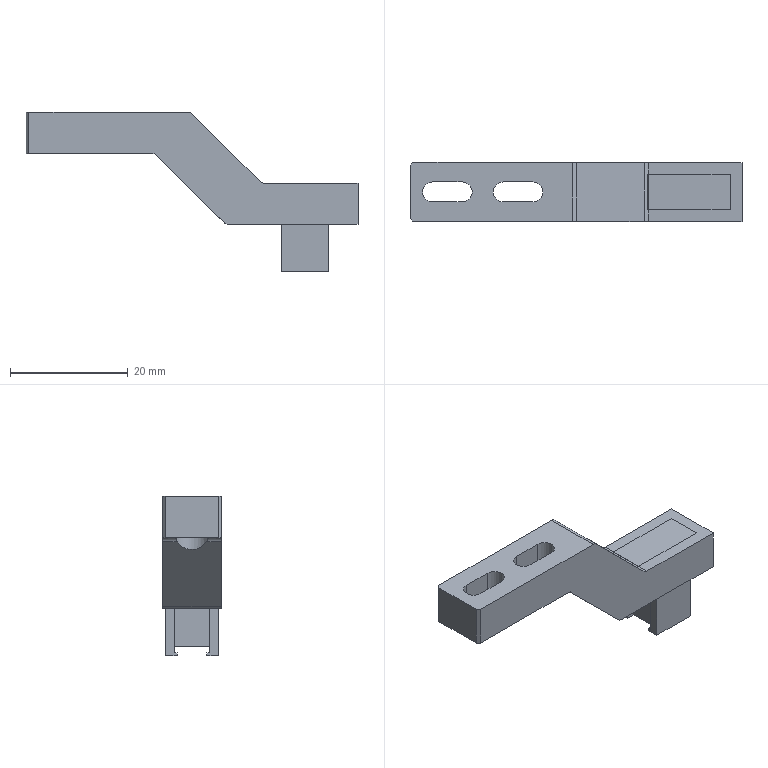Part | 2 solids | 62 faces | box 56.3 x 10 x 27 mm | volume 4591 mm3 | plane 48 | cylinder 14 | commonest cylinder face diameters 2 x6 3.4 x4 6 x4